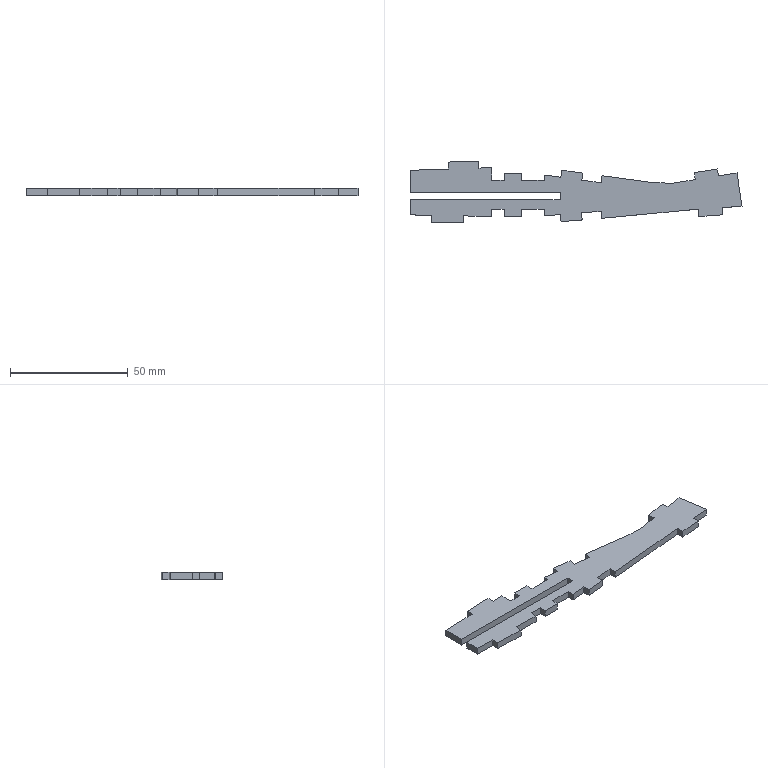Part | SolidWorks | features BaseBody 1 | 1 solid | 57 faces | box 140.807 x 26.276 x 3 mm | volume 6548 mm3 | plane 57